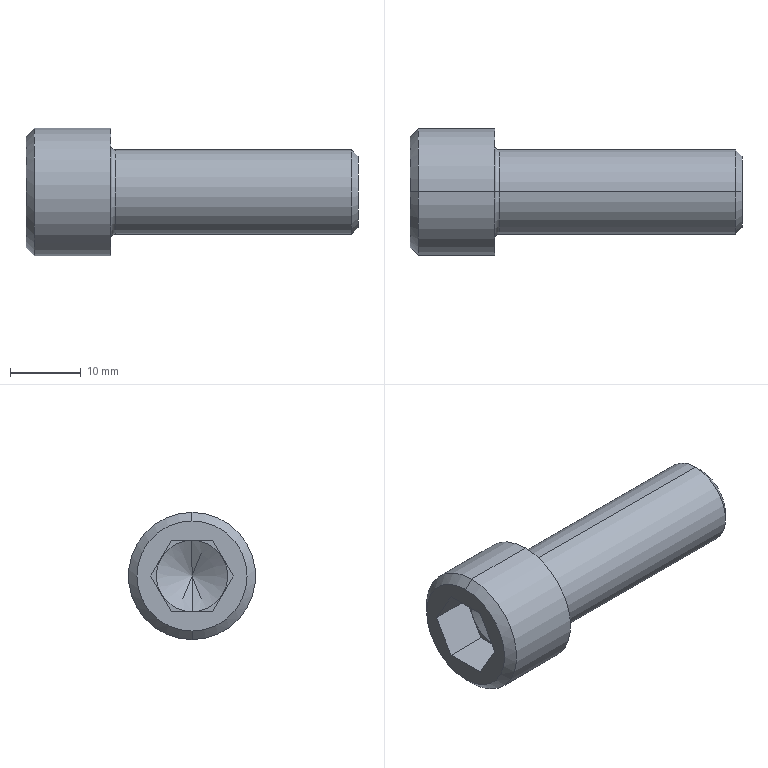Part | STEP file | socket head cap screw_am_B18.3.1M - 12 x 1.75 x 35 Hex SHCS -- 35NHX | 1 solid | 27 faces | box 47 x 18 x 18 mm | volume 6350 mm3 | plane 15 | cone 6 | cylinder 4 | torus 2 | commonest cylinder face diameters 12 x2 18 x2